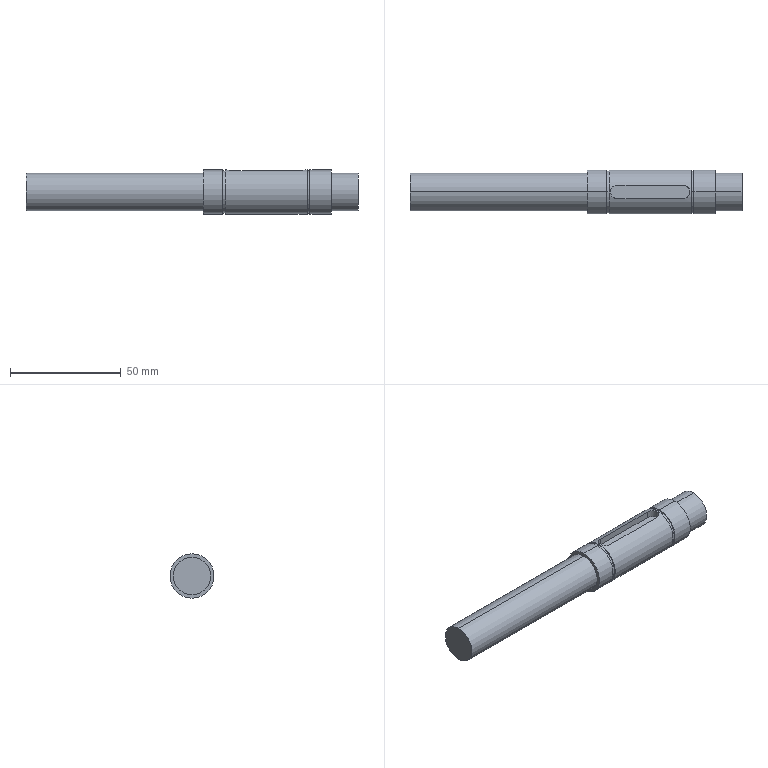Part | SolidWorks | features ICE 3, Extrusion 1, RevCut 1 | 1 solid | 28 faces | box 150 x 20 x 20 mm | volume 38325 mm3 | cylinder 17 | plane 11 | commonest cylinder face diameters 20 x6 17 x4 19 x4 6 x3
STEP:
#1=CARTESIAN_POINT('',(58.,0.,-10.));
#2=VERTEX_POINT('',#1);
#3=CARTESIAN_POINT('',(58.,0.,10.));
#4=VERTEX_POINT('',#3);
#5=CARTESIAN_POINT('',(58.,0.,0.));
#6=DIRECTION('',(1.,0.,0.));
#7=DIRECTION('',(0.,0.,-1.));
#8=AXIS2_PLACEMENT_3D('',#5,#6,#7);
#9=CIRCLE('',#8,10.);
#10=EDGE_CURVE('',#2,#4,#9,.T.);
#11=ORIENTED_EDGE('',*,*,#10,.F.);
#12=CARTESIAN_POINT('',(48.3,0.,-10.));
#13=VERTEX_POINT('',#12);
#14=CARTESIAN_POINT('',(58.,0.,-10.));
#15=DIRECTION('',(-1.,0.,0.));
#16=VECTOR('',#15,1000.);
#17=LINE('',#14,#16);
#18=EDGE_CURVE('',#2,#13,#17,.T.);
#19=ORIENTED_EDGE('',*,*,#18,.T.);
#20=CARTESIAN_POINT('',(48.3,0.,10.));
#21=VERTEX_POINT('',#20);
#22=CARTESIAN_POINT('',(48.3,0.,0.));
#23=DIRECTION('',(-1.,0.,0.));
#24=DIRECTION('',(0.,0.,1.));
#25=AXIS2_PLACEMENT_3D('',#22,#23,#24);
#26=CIRCLE('',#25,10.);
#27=EDGE_CURVE('',#21,#13,#26,.T.);
#28=ORIENTED_EDGE('',*,*,#27,.F.);
#29=CARTESIAN_POINT('',(58.,0.,10.));
#30=DIRECTION('',(-1.,0.,0.));
#31=VECTOR('',#30,1000.);
#32=LINE('',#29,#31);
#33=EDGE_CURVE('',#4,#21,#32,.T.);
#34=ORIENTED_EDGE('',*,*,#33,.F.);
#35=EDGE_LOOP('',(#11,#19,#28,#34));
#36=FACE_OUTER_BOUND('',#35,.T.);
#37=CARTESIAN_POINT('',(58.,0.,0.));
#38=DIRECTION('',(-1.,0.,0.));
#39=DIRECTION('',(0.,0.,1.));
#40=AXIS2_PLACEMENT_3D('',#37,#38,#39);
#41=CYLINDRICAL_SURFACE('',#40,10.);
#42=ADVANCED_FACE('',(#36),#41,.T.);
#43=CARTESIAN_POINT('',(70.,0.,-8.5));
#44=VERTEX_POINT('',#43);
#45=CARTESIAN_POINT('',(70.,0.,8.5));
#46=VERTEX_POINT('',#45);
#47=CARTESIAN_POINT('',(70.,0.,0.));
#48=DIRECTION('',(1.,0.,0.));
#49=DIRECTION('',(0.,0.,-1.));
#50=AXIS2_PLACEMENT_3D('',#47,#48,#49);
#51=CIRCLE('',#50,8.5);
#52=EDGE_CURVE('',#44,#46,#51,.T.);
#53=ORIENTED_EDGE('',*,*,#52,.F.);
#54=CARTESIAN_POINT('',(58.,0.,-8.5));
#55=VERTEX_POINT('',#54);
#56=CARTESIAN_POINT('',(70.,0.,-8.5));
#57=DIRECTION('',(-1.,0.,0.));
#58=VECTOR('',#57,1000.);
#59=LINE('',#56,#58);
#60=EDGE_CURVE('',#44,#55,#59,.T.);
#61=ORIENTED_EDGE('',*,*,#60,.T.);
#62=CARTESIAN_POINT('',(58.,0.,8.5));
#63=VERTEX_POINT('',#62);
#64=CARTESIAN_POINT('',(58.,0.,0.));
#65=DIRECTION('',(1.,0.,0.));
#66=DIRECTION('',(0.,0.,-1.));
#67=AXIS2_PLACEMENT_3D('',#64,#65,#66);
#68=CIRCLE('',#67,8.5);
#69=EDGE_CURVE('',#55,#63,#68,.T.);
#70=ORIENTED_EDGE('',*,*,#69,.T.);
#71=CARTESIAN_POINT('',(70.,0.,8.5));
#72=DIRECTION('',(-1.,0.,0.));
#73=VECTOR('',#72,1000.);
#74=LINE('',#71,#73);
#75=EDGE_CURVE('',#46,#63,#74,.T.);
#76=ORIENTED_EDGE('',*,*,#75,.F.);
#77=EDGE_LOOP('',(#53,#61,#70,#76));
#78=FACE_OUTER_BOUND('',#77,.T.);
#79=CARTESIAN_POINT('',(70.,0.,0.));
#80=DIRECTION('',(-1.,0.,0.));
#81=DIRECTION('',(0.,0.,1.));
#82=AXIS2_PLACEMENT_3D('',#79,#80,#81);
#83=CYLINDRICAL_SURFACE('',#82,8.5);
#84=ADVANCED_FACE('',(#78),#83,.T.);
#85=CARTESIAN_POINT('',(48.3,0.,9.5));
#86=VERTEX_POINT('',#85);
#87=CARTESIAN_POINT('',(48.3,0.,-9.5));
#88=VERTEX_POINT('',#87);
#89=CARTESIAN_POINT('',(48.3,0.,0.));
#90=DIRECTION('',(-1.,0.,0.));
#91=DIRECTION('',(0.,0.,1.));
#92=AXIS2_PLACEMENT_3D('',#89,#90,#91);
#93=CIRCLE('',#92,9.5);
#94=EDGE_CURVE('',#86,#88,#93,.T.);
#95=ORIENTED_EDGE('',*,*,#94,.T.);
#96=CARTESIAN_POINT('',(47.,0.,-9.5));
#97=VERTEX_POINT('',#96);
#98=CARTESIAN_POINT('',(0.,0.,-9.5));
#99=DIRECTION('',(-1.,0.,0.));
#100=VECTOR('',#99,1000.);
#101=LINE('',#98,#100);
#102=EDGE_CURVE('',#88,#97,#101,.T.);
#103=ORIENTED_EDGE('',*,*,#102,.T.);
#104=CARTESIAN_POINT('',(47.,0.,9.5));
#105=VERTEX_POINT('',#104);
#106=CARTESIAN_POINT('',(47.,0.,0.));
#107=DIRECTION('',(-1.,0.,0.));
#108=DIRECTION('',(0.,0.,1.));
#109=AXIS2_PLACEMENT_3D('',#106,#107,#108);
#110=CIRCLE('',#109,9.5);
#111=EDGE_CURVE('',#105,#97,#110,.T.);
#112=ORIENTED_EDGE('',*,*,#111,.F.);
#113=CARTESIAN_POINT('',(0.,0.,9.5));
#114=DIRECTION('',(-1.,0.,0.));
#115=VECTOR('',#114,1000.);
#116=LINE('',#113,#115);
#117=EDGE_CURVE('',#86,#105,#116,.T.);
#118=ORIENTED_EDGE('',*,*,#117,.F.);
#119=EDGE_LOOP('',(#95,#103,#112,#118));
#120=FACE_OUTER_BOUND('',#119,.T.);
#121=CARTESIAN_POINT('',(0.,0.,0.));
#122=DIRECTION('',(-1.,0.,0.));
#123=DIRECTION('',(0.,0.,1.));
#124=AXIS2_PLACEMENT_3D('',#121,#122,#123);
#125=CYLINDRICAL_SURFACE('',#124,9.5);
#126=ADVANCED_FACE('',(#120),#125,.T.);
#127=CARTESIAN_POINT('',(47.,0.,10.));
#128=VERTEX_POINT('',#127);
#129=CARTESIAN_POINT('',(47.,0.,-10.));
#130=VERTEX_POINT('',#129);
#131=CARTESIAN_POINT('',(47.,0.,0.));
#132=DIRECTION('',(-1.,0.,0.));
#133=DIRECTION('',(0.,0.,1.));
#134=AXIS2_PLACEMENT_3D('',#131,#132,#133);
#135=CIRCLE('',#134,10.);
#136=EDGE_CURVE('',#128,#130,#135,.T.);
#137=ORIENTED_EDGE('',*,*,#136,.T.);
#138=CARTESIAN_POINT('',(10.,0.,-10.));
#139=VERTEX_POINT('',#138);
#140=CARTESIAN_POINT('',(58.,0.,-10.));
#141=DIRECTION('',(-1.,0.,0.));
#142=VECTOR('',#141,1000.);
#143=LINE('',#140,#142);
#144=EDGE_CURVE('',#130,#139,#143,.T.);
#145=ORIENTED_EDGE('',*,*,#144,.T.);
#146=CARTESIAN_POINT('',(10.,0.,10.));
#147=VERTEX_POINT('',#146);
#148=CARTESIAN_POINT('',(10.,0.,0.));
#149=DIRECTION('',(-1.,0.,0.));
#150=DIRECTION('',(0.,0.,1.));
#151=AXIS2_PLACEMENT_3D('',#148,#149,#150);
#152=CIRCLE('',#151,10.);
#153=EDGE_CURVE('',#147,#139,#152,.T.);
#154=ORIENTED_EDGE('',*,*,#153,.F.);
#155=CARTESIAN_POINT('',(10.5,0.,10.));
#156=VERTEX_POINT('',#155);
#157=CARTESIAN_POINT('',(58.,0.,10.));
#158=DIRECTION('',(-1.,0.,0.));
#159=VECTOR('',#158,1000.);
#160=LINE('',#157,#159);
#161=EDGE_CURVE('',#156,#147,#160,.T.);
#162=ORIENTED_EDGE('',*,*,#161,.F.);
#163=CARTESIAN_POINT('',(13.5,3.,9.539));
#164=VERTEX_POINT('',#163);
#165=CARTESIAN_POINT('',(13.5,3.,9.539));
#166=CARTESIAN_POINT('',(13.3,3.,9.539));
#167=CARTESIAN_POINT('',(13.105,2.98,9.546));
#168=CARTESIAN_POINT('',(12.719,2.903,9.569));
#169=CARTESIAN_POINT('',(12.528,2.845,9.587));
#170=CARTESIAN_POINT('',(12.165,2.694,9.631));
#171=CARTESIAN_POINT('',(11.994,2.602,9.656));
#172=CARTESIAN_POINT('',(11.668,2.384,9.712));
#173=CARTESIAN_POINT('',(11.515,2.258,9.743));
#174=CARTESIAN_POINT('',(11.103,1.845,9.832));
#175=CARTESIAN_POINT('',(10.88,1.512,9.892));
#176=CARTESIAN_POINT('',(10.655,0.971,9.954));
#177=CARTESIAN_POINT('',(10.597,0.7806,9.971));
#178=CARTESIAN_POINT('',(10.519,0.3926,9.994));
#179=CARTESIAN_POINT('',(10.5,0.197,10.));
#180=CARTESIAN_POINT('',(10.5,0.,10.));
#181=B_SPLINE_CURVE_WITH_KNOTS('',3,(#165,#166,#167,#168,#169,#170,#171,#172,#173,#174,#175,#176,#177,#178,#179,#180),.UNSPECIFIED.,.F.,.F.,(4,2,2,2,2,2,2,4),(0.,0.0005898,0.00118,0.001769,0.002359,0.003539,0.004128,0.004718),.UNSPECIFIED.);
#182=EDGE_CURVE('',#164,#156,#181,.T.);
#183=ORIENTED_EDGE('',*,*,#182,.F.);
#184=CARTESIAN_POINT('',(43.5,3.,9.539));
#185=VERTEX_POINT('',#184);
#186=CARTESIAN_POINT('',(58.,3.,9.539));
#187=DIRECTION('',(-1.,0.,0.));
#188=VECTOR('',#187,1000.);
#189=LINE('',#186,#188);
#190=EDGE_CURVE('',#185,#164,#189,.T.);
#191=ORIENTED_EDGE('',*,*,#190,.F.);
#192=CARTESIAN_POINT('',(46.5,0.,10.));
#193=VERTEX_POINT('',#192);
#194=CARTESIAN_POINT('',(46.5,0.,10.));
#195=CARTESIAN_POINT('',(46.5,0.1968,10.));
#196=CARTESIAN_POINT('',(46.48,0.3967,9.994));
#197=CARTESIAN_POINT('',(46.403,0.7821,9.971));
#198=CARTESIAN_POINT('',(46.346,0.9695,9.955));
#199=CARTESIAN_POINT('',(46.194,1.334,9.912));
#200=CARTESIAN_POINT('',(46.101,1.507,9.887));
#201=CARTESIAN_POINT('',(45.884,1.831,9.832));
#202=CARTESIAN_POINT('',(45.759,1.983,9.802));
#203=CARTESIAN_POINT('',(45.483,2.26,9.742));
#204=CARTESIAN_POINT('',(45.333,2.383,9.713));
#205=CARTESIAN_POINT('',(45.009,2.6,9.657));
#206=CARTESIAN_POINT('',(44.833,2.694,9.63));
#207=CARTESIAN_POINT('',(44.472,2.845,9.587));
#208=CARTESIAN_POINT('',(44.285,2.902,9.57));
#209=CARTESIAN_POINT('',(43.899,2.98,9.546));
#210=CARTESIAN_POINT('',(43.699,3.,9.539));
#211=CARTESIAN_POINT('',(43.5,3.,9.539));
#212=B_SPLINE_CURVE_WITH_KNOTS('',3,(#194,#195,#196,#197,#198,#199,#200,#201,#202,#203,#204,#205,#206,#207,#208,#209,#210,#211),.UNSPECIFIED.,.F.,.F.,(4,2,2,2,2,2,2,2,4),(0.004718,0.005307,0.005896,0.006485,0.007074,0.007663,0.008252,0.008842,0.009431),.UNSPECIFIED.);
#213=EDGE_CURVE('',#193,#185,#212,.T.);
#214=ORIENTED_EDGE('',*,*,#213,.F.);
#215=CARTESIAN_POINT('',(58.,0.,10.));
#216=DIRECTION('',(-1.,0.,0.));
#217=VECTOR('',#216,1000.);
#218=LINE('',#215,#217);
#219=EDGE_CURVE('',#128,#193,#218,.T.);
#220=ORIENTED_EDGE('',*,*,#219,.F.);
#221=EDGE_LOOP('',(#137,#145,#154,#162,#183,#191,#214,#220));
#222=FACE_OUTER_BOUND('',#221,.T.);
#223=CARTESIAN_POINT('',(58.,0.,0.));
#224=DIRECTION('',(-1.,0.,0.));
#225=DIRECTION('',(0.,0.,1.));
#226=AXIS2_PLACEMENT_3D('',#223,#224,#225);
#227=CYLINDRICAL_SURFACE('',#226,10.);
#228=ADVANCED_FACE('',(#222),#227,.T.);
#229=ORIENTED_EDGE('',*,*,#182,.T.);
#230=CARTESIAN_POINT('',(10.5,0.,6.5));
#231=VERTEX_POINT('',#230);
#232=CARTESIAN_POINT('',(10.5,0.,10.));
#233=DIRECTION('',(0.,0.,-1.));
#234=VECTOR('',#233,1000.);
#235=LINE('',#232,#234);
#236=EDGE_CURVE('',#156,#231,#235,.T.);
#237=ORIENTED_EDGE('',*,*,#236,.T.);
#238=CARTESIAN_POINT('',(13.5,3.,6.5));
#239=VERTEX_POINT('',#238);
#240=CARTESIAN_POINT('',(13.5,0.,6.5));
#241=DIRECTION('',(0.,0.,1.));
#242=DIRECTION('',(1.,0.,0.));
#243=AXIS2_PLACEMENT_3D('',#240,#241,#242);
#244=CIRCLE('',#243,3.);
#245=EDGE_CURVE('',#239,#231,#244,.T.);
#246=ORIENTED_EDGE('',*,*,#245,.F.);
#247=CARTESIAN_POINT('',(13.5,3.,10.));
#248=DIRECTION('',(0.,0.,-1.));
#249=VECTOR('',#248,1000.);
#250=LINE('',#247,#249);
#251=EDGE_CURVE('',#164,#239,#250,.T.);
#252=ORIENTED_EDGE('',*,*,#251,.F.);
#253=EDGE_LOOP('',(#229,#237,#246,#252));
#254=FACE_OUTER_BOUND('',#253,.T.);
#255=CARTESIAN_POINT('',(13.5,0.,10.));
#256=DIRECTION('',(0.,0.,-1.));
#257=DIRECTION('',(-1.,0.,0.));
#258=AXIS2_PLACEMENT_3D('',#255,#256,#257);
#259=CYLINDRICAL_SURFACE('',#258,3.);
#260=ADVANCED_FACE('',(#254),#259,.F.);
#261=CARTESIAN_POINT('',(10.,0.,9.5));
#262=VERTEX_POINT('',#261);
#263=CARTESIAN_POINT('',(10.,0.,-9.5));
#264=VERTEX_POINT('',#263);
#265=CARTESIAN_POINT('',(10.,0.,0.));
#266=DIRECTION('',(-1.,0.,0.));
#267=DIRECTION('',(0.,0.,1.));
#268=AXIS2_PLACEMENT_3D('',#265,#266,#267);
#269=CIRCLE('',#268,9.5);
#270=EDGE_CURVE('',#262,#264,#269,.T.);
#271=ORIENTED_EDGE('',*,*,#270,.T.);
#272=CARTESIAN_POINT('',(8.7,0.,-9.5));
#273=VERTEX_POINT('',#272);
#274=CARTESIAN_POINT('',(0.,0.,-9.5));
#275=DIRECTION('',(-1.,0.,0.));
#276=VECTOR('',#275,1000.);
#277=LINE('',#274,#276);
#278=EDGE_CURVE('',#264,#273,#277,.T.);
#279=ORIENTED_EDGE('',*,*,#278,.T.);
#280=CARTESIAN_POINT('',(8.7,0.,9.5));
#281=VERTEX_POINT('',#280);
#282=CARTESIAN_POINT('',(8.7,0.,0.));
#283=DIRECTION('',(-1.,0.,0.));
#284=DIRECTION('',(0.,0.,1.));
#285=AXIS2_PLACEMENT_3D('',#282,#283,#284);
#286=CIRCLE('',#285,9.5);
#287=EDGE_CURVE('',#281,#273,#286,.T.);
#288=ORIENTED_EDGE('',*,*,#287,.F.);
#289=CARTESIAN_POINT('',(0.,0.,9.5));
#290=DIRECTION('',(-1.,0.,0.));
#291=VECTOR('',#290,1000.);
#292=LINE('',#289,#291);
#293=EDGE_CURVE('',#262,#281,#292,.T.);
#294=ORIENTED_EDGE('',*,*,#293,.F.);
#295=EDGE_LOOP('',(#271,#279,#288,#294));
#296=FACE_OUTER_BOUND('',#295,.T.);
#297=CARTESIAN_POINT('',(0.,0.,0.));
#298=DIRECTION('',(-1.,0.,0.));
#299=DIRECTION('',(0.,0.,1.));
#300=AXIS2_PLACEMENT_3D('',#297,#298,#299);
#301=CYLINDRICAL_SURFACE('',#300,9.5);
#302=ADVANCED_FACE('',(#296),#301,.T.);
#303=CARTESIAN_POINT('',(-80.,0.,8.5));
#304=VERTEX_POINT('',#303);
#305=CARTESIAN_POINT('',(-80.,0.,-8.5));
#306=VERTEX_POINT('',#305);
#307=CARTESIAN_POINT('',(-80.,0.,0.));
#308=DIRECTION('',(-1.,0.,0.));
#309=DIRECTION('',(0.,0.,1.));
#310=AXIS2_PLACEMENT_3D('',#307,#308,#309);
#311=CIRCLE('',#310,8.5);
#312=EDGE_CURVE('',#304,#306,#311,.T.);
#313=ORIENTED_EDGE('',*,*,#312,.F.);
#314=CARTESIAN_POINT('',(0.,0.,8.5));
#315=VERTEX_POINT('',#314);
#316=CARTESIAN_POINT('',(-80.,0.,8.5));
#317=DIRECTION('',(1.,0.,0.));
#318=VECTOR('',#317,1000.);
#319=LINE('',#316,#318);
#320=EDGE_CURVE('',#304,#315,#319,.T.);
#321=ORIENTED_EDGE('',*,*,#320,.T.);
#322=CARTESIAN_POINT('',(0.,0.,-8.5));
#323=VERTEX_POINT('',#322);
#324=CARTESIAN_POINT('',(0.,0.,0.));
#325=DIRECTION('',(-1.,0.,0.));
#326=DIRECTION('',(0.,0.,1.));
#327=AXIS2_PLACEMENT_3D('',#324,#325,#326);
#328=CIRCLE('',#327,8.5);
#329=EDGE_CURVE('',#315,#323,#328,.T.);
#330=ORIENTED_EDGE('',*,*,#329,.T.);
#331=CARTESIAN_POINT('',(-80.,0.,-8.5));
#332=DIRECTION('',(1.,0.,0.));
#333=VECTOR('',#332,1000.);
#334=LINE('',#331,#333);
#335=EDGE_CURVE('',#306,#323,#334,.T.);
#336=ORIENTED_EDGE('',*,*,#335,.F.);
#337=EDGE_LOOP('',(#313,#321,#330,#336));
#338=FACE_OUTER_BOUND('',#337,.T.);
#339=CARTESIAN_POINT('',(-80.,0.,0.));
#340=DIRECTION('',(1.,0.,0.));
#341=DIRECTION('',(0.,0.,-1.));
#342=AXIS2_PLACEMENT_3D('',#339,#340,#341);
#343=CYLINDRICAL_SURFACE('',#342,8.5);
#344=ADVANCED_FACE('',(#338),#343,.T.);
#345=CARTESIAN_POINT('',(8.7,0.,10.));
#346=VERTEX_POINT('',#345);
#347=CARTESIAN_POINT('',(8.7,0.,-10.));
#348=VERTEX_POINT('',#347);
#349=CARTESIAN_POINT('',(8.7,0.,0.));
#350=DIRECTION('',(-1.,0.,0.));
#351=DIRECTION('',(0.,0.,1.));
#352=AXIS2_PLACEMENT_3D('',#349,#350,#351);
#353=CIRCLE('',#352,10.);
#354=EDGE_CURVE('',#346,#348,#353,.T.);
#355=ORIENTED_EDGE('',*,*,#354,.T.);
#356=CARTESIAN_POINT('',(0.,0.,-10.));
#357=VERTEX_POINT('',#356);
#358=CARTESIAN_POINT('',(58.,0.,-10.));
#359=DIRECTION('',(-1.,0.,0.));
#360=VECTOR('',#359,1000.);
#361=LINE('',#358,#360);
#362=EDGE_CURVE('',#348,#357,#361,.T.);
#363=ORIENTED_EDGE('',*,*,#362,.T.);
#364=CARTESIAN_POINT('',(0.,0.,10.));
#365=VERTEX_POINT('',#364);
#366=CARTESIAN_POINT('',(0.,0.,0.));
#367=DIRECTION('',(1.,0.,0.));
#368=DIRECTION('',(0.,0.,-1.));
#369=AXIS2_PLACEMENT_3D('',#366,#367,#368);
#370=CIRCLE('',#369,10.);
#371=EDGE_CURVE('',#357,#365,#370,.T.);
#372=ORIENTED_EDGE('',*,*,#371,.T.);
#373=CARTESIAN_POINT('',(58.,0.,10.));
#374=DIRECTION('',(-1.,0.,0.));
#375=VECTOR('',#374,1000.);
#376=LINE('',#373,#375);
#377=EDGE_CURVE('',#346,#365,#376,.T.);
#378=ORIENTED_EDGE('',*,*,#377,.F.);
#379=EDGE_LOOP('',(#355,#363,#372,#378));
#380=FACE_OUTER_BOUND('',#379,.T.);
#381=CARTESIAN_POINT('',(58.,0.,0.));
#382=DIRECTION('',(-1.,0.,0.));
#383=DIRECTION('',(0.,0.,1.));
#384=AXIS2_PLACEMENT_3D('',#381,#382,#383);
#385=CYLINDRICAL_SURFACE('',#384,10.);
#386=ADVANCED_FACE('',(#380),#385,.T.);
#387=ORIENTED_EDGE('',*,*,#362,.F.);
#388=CARTESIAN_POINT('',(8.7,0.,0.));
#389=DIRECTION('',(-1.,0.,0.));
#390=DIRECTION('',(0.,0.,1.));
#391=AXIS2_PLACEMENT_3D('',#388,#389,#390);
#392=CIRCLE('',#391,10.);
#393=EDGE_CURVE('',#348,#346,#392,.T.);
#394=ORIENTED_EDGE('',*,*,#393,.T.);
#395=ORIENTED_EDGE('',*,*,#377,.T.);
#396=CARTESIAN_POINT('',(0.,0.,0.));
#397=DIRECTION('',(1.,0.,0.));
#398=DIRECTION('',(0.,0.,-1.));
#399=AXIS2_PLACEMENT_3D('',#396,#397,#398);
#400=CIRCLE('',#399,10.);
#401=EDGE_CURVE('',#365,#357,#400,.T.);
#402=ORIENTED_EDGE('',*,*,#401,.T.);
#403=EDGE_LOOP('',(#387,#394,#395,#402));
#404=FACE_OUTER_BOUND('',#403,.T.);
#405=CARTESIAN_POINT('',(58.,0.,0.));
#406=DIRECTION('',(-1.,0.,0.));
#407=DIRECTION('',(0.,0.,1.));
#408=AXIS2_PLACEMENT_3D('',#405,#406,#407);
#409=CYLINDRICAL_SURFACE('',#408,10.);
#410=ADVANCED_FACE('',(#404),#409,.T.);
#411=CARTESIAN_POINT('',(0.,0.,0.));
#412=DIRECTION('',(-1.,0.,0.));
#413=DIRECTION('',(0.,0.,1.));
#414=AXIS2_PLACEMENT_3D('',#411,#412,#413);
#415=CIRCLE('',#414,8.5);
#416=EDGE_CURVE('',#323,#315,#415,.T.);
#417=ORIENTED_EDGE('',*,*,#416,.F.);
#418=ORIENTED_EDGE('',*,*,#329,.F.);
#419=EDGE_LOOP('',(#417,#418));
#420=FACE_BOUND('',#419,.T.);
#421=ORIENTED_EDGE('',*,*,#401,.F.);
#422=ORIENTED_EDGE('',*,*,#371,.F.);
#423=EDGE_LOOP('',(#421,#422));
#424=FACE_OUTER_BOUND('',#423,.T.);
#425=CARTESIAN_POINT('',(0.,0.,0.));
#426=DIRECTION('',(1.,0.,0.));
#427=DIRECTION('',(0.,0.,-1.));
#428=AXIS2_PLACEMENT_3D('',#425,#426,#427);
#429=PLANE('',#428);
#430=ADVANCED_FACE('',(#420,#424),#429,.F.);
#431=ORIENTED_EDGE('',*,*,#320,.F.);
#432=CARTESIAN_POINT('',(-80.,0.,0.));
#433=DIRECTION('',(-1.,0.,0.));
#434=DIRECTION('',(0.,0.,1.));
#435=AXIS2_PLACEMENT_3D('',#432,#433,#434);
#436=CIRCLE('',#435,8.5);
#437=EDGE_CURVE('',#306,#304,#436,.T.);
#438=ORIENTED_EDGE('',*,*,#437,.F.);
#439=ORIENTED_EDGE('',*,*,#335,.T.);
#440=ORIENTED_EDGE('',*,*,#416,.T.);
#441=EDGE_LOOP('',(#431,#438,#439,#440));
#442=FACE_OUTER_BOUND('',#441,.T.);
#443=CARTESIAN_POINT('',(-80.,0.,0.));
#444=DIRECTION('',(1.,0.,0.));
#445=DIRECTION('',(0.,0.,-1.));
#446=AXIS2_PLACEMENT_3D('',#443,#444,#445);
#447=CYLINDRICAL_SURFACE('',#446,8.5);
#448=ADVANCED_FACE('',(#442),#447,.T.);
#449=ORIENTED_EDGE('',*,*,#437,.T.);
#450=ORIENTED_EDGE('',*,*,#312,.T.);
#451=EDGE_LOOP('',(#449,#450));
#452=FACE_OUTER_BOUND('',#451,.T.);
#453=CARTESIAN_POINT('',(-80.,0.,0.));
#454=DIRECTION('',(-1.,0.,0.));
#455=DIRECTION('',(0.,0.,1.));
#456=AXIS2_PLACEMENT_3D('',#453,#454,#455);
#457=PLANE('',#456);
#458=ADVANCED_FACE('',(#452),#457,.T.);
#459=ORIENTED_EDGE('',*,*,#287,.T.);
#460=CARTESIAN_POINT('',(8.7,0.,0.));
#461=DIRECTION('',(-1.,0.,0.));
#462=DIRECTION('',(0.,0.,1.));
#463=AXIS2_PLACEMENT_3D('',#460,#461,#462);
#464=CIRCLE('',#463,9.5);
#465=EDGE_CURVE('',#273,#281,#464,.T.);
#466=ORIENTED_EDGE('',*,*,#465,.T.);
#467=EDGE_LOOP('',(#459,#466));
#468=FACE_BOUND('',#467,.T.);
#469=ORIENTED_EDGE('',*,*,#354,.F.);
#470=ORIENTED_EDGE('',*,*,#393,.F.);
#471=EDGE_LOOP('',(#469,#470));
#472=FACE_OUTER_BOUND('',#471,.T.);
#473=CARTESIAN_POINT('',(8.7,0.,-10.));
#474=DIRECTION('',(1.,0.,0.));
#475=DIRECTION('',(0.,0.,-1.));
#476=AXIS2_PLACEMENT_3D('',#473,#474,#475);
#477=PLANE('',#476);
#478=ADVANCED_FACE('',(#468,#472),#477,.T.);
#479=ORIENTED_EDGE('',*,*,#278,.F.);
#480=CARTESIAN_POINT('',(10.,0.,0.));
#481=DIRECTION('',(-1.,0.,0.));
#482=DIRECTION('',(0.,0.,1.));
#483=AXIS2_PLACEMENT_3D('',#480,#481,#482);
#484=CIRCLE('',#483,9.5);
#485=EDGE_CURVE('',#264,#262,#484,.T.);
#486=ORIENTED_EDGE('',*,*,#485,.T.);
#487=ORIENTED_EDGE('',*,*,#293,.T.);
#488=ORIENTED_EDGE('',*,*,#465,.F.);
#489=EDGE_LOOP('',(#479,#486,#487,#488));
#490=FACE_OUTER_BOUND('',#489,.T.);
#491=CARTESIAN_POINT('',(0.,0.,0.));
#492=DIRECTION('',(-1.,0.,0.));
#493=DIRECTION('',(0.,0.,1.));
#494=AXIS2_PLACEMENT_3D('',#491,#492,#493);
#495=CYLINDRICAL_SURFACE('',#494,9.5);
#496=ADVANCED_FACE('',(#490),#495,.T.);
#497=ORIENTED_EDGE('',*,*,#153,.T.);
#498=CARTESIAN_POINT('',(10.,0.,0.));
#499=DIRECTION('',(-1.,0.,0.));
#500=DIRECTION('',(0.,0.,1.));
#501=AXIS2_PLACEMENT_3D('',#498,#499,#500);
#502=CIRCLE('',#501,10.);
#503=EDGE_CURVE('',#139,#147,#502,.T.);
#504=ORIENTED_EDGE('',*,*,#503,.T.);
#505=EDGE_LOOP('',(#497,#504));
#506=FACE_OUTER_BOUND('',#505,.T.);
#507=ORIENTED_EDGE('',*,*,#270,.F.);
#508=ORIENTED_EDGE('',*,*,#485,.F.);
#509=EDGE_LOOP('',(#507,#508));
#510=FACE_BOUND('',#509,.T.);
#511=CARTESIAN_POINT('',(10.,0.,-10.));
#512=DIRECTION('',(-1.,0.,0.));
#513=DIRECTION('',(0.,0.,1.));
#514=AXIS2_PLACEMENT_3D('',#511,#512,#513);
#515=PLANE('',#514);
#516=ADVANCED_FACE('',(#506,#510),#515,.T.);
#517=ORIENTED_EDGE('',*,*,#245,.T.);
#518=CARTESIAN_POINT('',(13.5,-3.,6.5));
#519=VERTEX_POINT('',#518);
#520=CARTESIAN_POINT('',(13.5,0.,6.5));
#521=DIRECTION('',(0.,0.,1.));
#522=DIRECTION('',(1.,0.,0.));
#523=AXIS2_PLACEMENT_3D('',#520,#521,#522);
#524=CIRCLE('',#523,3.);
#525=EDGE_CURVE('',#231,#519,#524,.T.);
#526=ORIENTED_EDGE('',*,*,#525,.T.);
#527=CARTESIAN_POINT('',(43.5,-3.,6.5));
#528=VERTEX_POINT('',#527);
#529=CARTESIAN_POINT('',(13.5,-3.,6.5));
#530=DIRECTION('',(1.,0.,0.));
#531=VECTOR('',#530,1000.);
#532=LINE('',#529,#531);
#533=EDGE_CURVE('',#519,#528,#532,.T.);
#534=ORIENTED_EDGE('',*,*,#533,.T.);
#535=CARTESIAN_POINT('',(43.5,3.,6.5));
#536=VERTEX_POINT('',#535);
#537=CARTESIAN_POINT('',(43.5,0.,6.5));
#538=DIRECTION('',(0.,0.,1.));
#539=DIRECTION('',(1.,0.,0.));
#540=AXIS2_PLACEMENT_3D('',#537,#538,#539);
#541=CIRCLE('',#540,3.);
#542=EDGE_CURVE('',#528,#536,#541,.T.);
#543=ORIENTED_EDGE('',*,*,#542,.T.);
#544=CARTESIAN_POINT('',(13.5,3.,6.5));
#545=DIRECTION('',(-1.,0.,0.));
#546=VECTOR('',#545,1000.);
#547=LINE('',#544,#546);
#548=EDGE_CURVE('',#536,#239,#547,.T.);
#549=ORIENTED_EDGE('',*,*,#548,.T.);
#550=EDGE_LOOP('',(#517,#526,#534,#543,#549));
#551=FACE_OUTER_BOUND('',#550,.T.);
#552=CARTESIAN_POINT('',(13.5,0.,6.5));
#553=DIRECTION('',(0.,0.,1.));
#554=DIRECTION('',(1.,0.,0.));
#555=AXIS2_PLACEMENT_3D('',#552,#553,#554);
#556=PLANE('',#555);
#557=ADVANCED_FACE('',(#551),#556,.T.);
#558=ORIENTED_EDGE('',*,*,#190,.T.);
#559=ORIENTED_EDGE('',*,*,#251,.T.);
#560=ORIENTED_EDGE('',*,*,#548,.F.);
#561=CARTESIAN_POINT('',(43.5,3.,10.));
#562=DIRECTION('',(0.,0.,-1.));
#563=VECTOR('',#562,1000.);
#564=LINE('',#561,#563);
#565=EDGE_CURVE('',#185,#536,#564,.T.);
#566=ORIENTED_EDGE('',*,*,#565,.F.);
#567=EDGE_LOOP('',(#558,#559,#560,#566));
#568=FACE_OUTER_BOUND('',#567,.T.);
#569=CARTESIAN_POINT('',(13.5,3.,10.));
#570=DIRECTION('',(0.,-1.,0.));
#571=DIRECTION('',(1.,0.,0.));
#572=AXIS2_PLACEMENT_3D('',#569,#570,#571);
#573=PLANE('',#572);
#574=ADVANCED_FACE('',(#568),#573,.T.);
#575=ORIENTED_EDGE('',*,*,#236,.F.);
#576=CARTESIAN_POINT('',(13.5,-3.,9.539));
#577=VERTEX_POINT('',#576);
#578=CARTESIAN_POINT('',(10.5,0.,10.));
#579=CARTESIAN_POINT('',(10.5,-0.1968,10.));
#580=CARTESIAN_POINT('',(10.52,-0.3967,9.994));
#581=CARTESIAN_POINT('',(10.597,-0.7821,9.971));
#582=CARTESIAN_POINT('',(10.654,-0.9695,9.955));
#583=CARTESIAN_POINT('',(10.806,-1.334,9.912));
#584=CARTESIAN_POINT('',(10.899,-1.507,9.887));
#585=CARTESIAN_POINT('',(11.116,-1.831,9.832));
#586=CARTESIAN_POINT('',(11.241,-1.983,9.802));
#587=CARTESIAN_POINT('',(11.517,-2.26,9.742));
#588=CARTESIAN_POINT('',(11.667,-2.383,9.713));
#589=CARTESIAN_POINT('',(11.991,-2.6,9.657));
#590=CARTESIAN_POINT('',(12.167,-2.694,9.63));
#591=CARTESIAN_POINT('',(12.528,-2.845,9.587));
#592=CARTESIAN_POINT('',(12.715,-2.902,9.57));
#593=CARTESIAN_POINT('',(13.101,-2.98,9.546));
#594=CARTESIAN_POINT('',(13.301,-3.,9.539));
#595=CARTESIAN_POINT('',(13.5,-3.,9.539));
#596=B_SPLINE_CURVE_WITH_KNOTS('',3,(#578,#579,#580,#581,#582,#583,#584,#585,#586,#587,#588,#589,#590,#591,#592,#593,#594,#595),.UNSPECIFIED.,.F.,.F.,(4,2,2,2,2,2,2,2,4),(0.004718,0.005307,0.005896,0.006485,0.007074,0.007663,0.008252,0.008842,0.009431),.UNSPECIFIED.);
#597=EDGE_CURVE('',#156,#577,#596,.T.);
#598=ORIENTED_EDGE('',*,*,#597,.T.);
#599=CARTESIAN_POINT('',(13.5,-3.,10.));
#600=DIRECTION('',(0.,0.,-1.));
#601=VECTOR('',#600,1000.);
#602=LINE('',#599,#601);
#603=EDGE_CURVE('',#577,#519,#602,.T.);
#604=ORIENTED_EDGE('',*,*,#603,.T.);
#605=ORIENTED_EDGE('',*,*,#525,.F.);
#606=EDGE_LOOP('',(#575,#598,#604,#605));
#607=FACE_OUTER_BOUND('',#606,.T.);
#608=CARTESIAN_POINT('',(13.5,0.,10.));
#609=DIRECTION('',(0.,0.,-1.));
#610=DIRECTION('',(-1.,0.,0.));
#611=AXIS2_PLACEMENT_3D('',#608,#609,#610);
#612=CYLINDRICAL_SURFACE('',#611,3.);
#613=ADVANCED_FACE('',(#607),#612,.F.);
#614=CARTESIAN_POINT('',(43.5,-3.,9.539));
#615=VERTEX_POINT('',#614);
#616=CARTESIAN_POINT('',(58.,-3.,9.539));
#617=DIRECTION('',(1.,0.,0.));
#618=VECTOR('',#617,1000.);
#619=LINE('',#616,#618);
#620=EDGE_CURVE('',#577,#615,#619,.T.);
#621=ORIENTED_EDGE('',*,*,#620,.T.);
#622=CARTESIAN_POINT('',(43.5,-3.,10.));
#623=DIRECTION('',(0.,0.,-1.));
#624=VECTOR('',#623,1000.);
#625=LINE('',#622,#624);
#626=EDGE_CURVE('',#615,#528,#625,.T.);
#627=ORIENTED_EDGE('',*,*,#626,.T.);
#628=ORIENTED_EDGE('',*,*,#533,.F.);
#629=ORIENTED_EDGE('',*,*,#603,.F.);
#630=EDGE_LOOP('',(#621,#627,#628,#629));
#631=FACE_OUTER_BOUND('',#630,.T.);
#632=CARTESIAN_POINT('',(13.5,-3.,10.));
#633=DIRECTION('',(0.,1.,0.));
#634=DIRECTION('',(-1.,0.,0.));
#635=AXIS2_PLACEMENT_3D('',#632,#633,#634);
#636=PLANE('',#635);
#637=ADVANCED_FACE('',(#631),#636,.T.);
#638=ORIENTED_EDGE('',*,*,#626,.F.);
#639=CARTESIAN_POINT('',(43.5,-3.,9.539));
#640=CARTESIAN_POINT('',(43.7,-3.,9.539));
#641=CARTESIAN_POINT('',(43.895,-2.98,9.546));
#642=CARTESIAN_POINT('',(44.281,-2.903,9.569));
#643=CARTESIAN_POINT('',(44.472,-2.845,9.587));
#644=CARTESIAN_POINT('',(44.835,-2.694,9.631));
#645=CARTESIAN_POINT('',(45.006,-2.602,9.656));
#646=CARTESIAN_POINT('',(45.332,-2.384,9.712));
#647=CARTESIAN_POINT('',(45.485,-2.258,9.743));
#648=CARTESIAN_POINT('',(45.897,-1.845,9.832));
#649=CARTESIAN_POINT('',(46.12,-1.512,9.892));
#650=CARTESIAN_POINT('',(46.345,-0.971,9.954));
#651=CARTESIAN_POINT('',(46.403,-0.7806,9.971));
#652=CARTESIAN_POINT('',(46.481,-0.3926,9.994));
#653=CARTESIAN_POINT('',(46.5,-0.197,10.));
#654=CARTESIAN_POINT('',(46.5,0.,10.));
#655=B_SPLINE_CURVE_WITH_KNOTS('',3,(#639,#640,#641,#642,#643,#644,#645,#646,#647,#648,#649,#650,#651,#652,#653,#654),.UNSPECIFIED.,.F.,.F.,(4,2,2,2,2,2,2,4),(0.,0.0005898,0.00118,0.001769,0.002359,0.003539,0.004128,0.004718),.UNSPECIFIED.);
#656=EDGE_CURVE('',#615,#193,#655,.T.);
#657=ORIENTED_EDGE('',*,*,#656,.T.);
#658=ORIENTED_EDGE('',*,*,#213,.T.);
#659=ORIENTED_EDGE('',*,*,#565,.T.);
#660=ORIENTED_EDGE('',*,*,#542,.F.);
#661=EDGE_LOOP('',(#638,#657,#658,#659,#660));
#662=FACE_OUTER_BOUND('',#661,.T.);
#663=CARTESIAN_POINT('',(43.5,0.,10.));
#664=DIRECTION('',(0.,0.,-1.));
#665=DIRECTION('',(-1.,0.,0.));
#666=AXIS2_PLACEMENT_3D('',#663,#664,#665);
#667=CYLINDRICAL_SURFACE('',#666,3.);
#668=ADVANCED_FACE('',(#662),#667,.F.);
#669=ORIENTED_EDGE('',*,*,#144,.F.);
#670=CARTESIAN_POINT('',(47.,0.,0.));
#671=DIRECTION('',(-1.,0.,0.));
#672=DIRECTION('',(0.,0.,1.));
#673=AXIS2_PLACEMENT_3D('',#670,#671,#672);
#674=CIRCLE('',#673,10.);
#675=EDGE_CURVE('',#130,#128,#674,.T.);
#676=ORIENTED_EDGE('',*,*,#675,.T.);
#677=ORIENTED_EDGE('',*,*,#219,.T.);
#678=ORIENTED_EDGE('',*,*,#656,.F.);
#679=ORIENTED_EDGE('',*,*,#620,.F.);
#680=ORIENTED_EDGE('',*,*,#597,.F.);
#681=ORIENTED_EDGE('',*,*,#161,.T.);
#682=ORIENTED_EDGE('',*,*,#503,.F.);
#683=EDGE_LOOP('',(#669,#676,#677,#678,#679,#680,#681,#682));
#684=FACE_OUTER_BOUND('',#683,.T.);
#685=CARTESIAN_POINT('',(58.,0.,0.));
#686=DIRECTION('',(-1.,0.,0.));
#687=DIRECTION('',(0.,0.,1.));
#688=AXIS2_PLACEMENT_3D('',#685,#686,#687);
#689=CYLINDRICAL_SURFACE('',#688,10.);
#690=ADVANCED_FACE('',(#684),#689,.T.);
#691=ORIENTED_EDGE('',*,*,#111,.T.);
#692=CARTESIAN_POINT('',(47.,0.,0.));
#693=DIRECTION('',(-1.,0.,0.));
#694=DIRECTION('',(0.,0.,1.));
#695=AXIS2_PLACEMENT_3D('',#692,#693,#694);
#696=CIRCLE('',#695,9.5);
#697=EDGE_CURVE('',#97,#105,#696,.T.);
#698=ORIENTED_EDGE('',*,*,#697,.T.);
#699=EDGE_LOOP('',(#691,#698));
#700=FACE_BOUND('',#699,.T.);
#701=ORIENTED_EDGE('',*,*,#136,.F.);
#702=ORIENTED_EDGE('',*,*,#675,.F.);
#703=EDGE_LOOP('',(#701,#702));
#704=FACE_OUTER_BOUND('',#703,.T.);
#705=CARTESIAN_POINT('',(47.,0.,-10.));
#706=DIRECTION('',(1.,0.,0.));
#707=DIRECTION('',(0.,0.,-1.));
#708=AXIS2_PLACEMENT_3D('',#705,#706,#707);
#709=PLANE('',#708);
#710=ADVANCED_FACE('',(#700,#704),#709,.T.);
#711=ORIENTED_EDGE('',*,*,#102,.F.);
#712=CARTESIAN_POINT('',(48.3,0.,0.));
#713=DIRECTION('',(-1.,0.,0.));
#714=DIRECTION('',(0.,0.,1.));
#715=AXIS2_PLACEMENT_3D('',#712,#713,#714);
#716=CIRCLE('',#715,9.5);
#717=EDGE_CURVE('',#88,#86,#716,.T.);
#718=ORIENTED_EDGE('',*,*,#717,.T.);
#719=ORIENTED_EDGE('',*,*,#117,.T.);
#720=ORIENTED_EDGE('',*,*,#697,.F.);
#721=EDGE_LOOP('',(#711,#718,#719,#720));
#722=FACE_OUTER_BOUND('',#721,.T.);
#723=CARTESIAN_POINT('',(0.,0.,0.));
#724=DIRECTION('',(-1.,0.,0.));
#725=DIRECTION('',(0.,0.,1.));
#726=AXIS2_PLACEMENT_3D('',#723,#724,#725);
#727=CYLINDRICAL_SURFACE('',#726,9.5);
#728=ADVANCED_FACE('',(#722),#727,.T.);
#729=ORIENTED_EDGE('',*,*,#27,.T.);
#730=CARTESIAN_POINT('',(48.3,0.,0.));
#731=DIRECTION('',(-1.,0.,0.));
#732=DIRECTION('',(0.,0.,1.));
#733=AXIS2_PLACEMENT_3D('',#730,#731,#732);
#734=CIRCLE('',#733,10.);
#735=EDGE_CURVE('',#13,#21,#734,.T.);
#736=ORIENTED_EDGE('',*,*,#735,.T.);
#737=EDGE_LOOP('',(#729,#736));
#738=FACE_OUTER_BOUND('',#737,.T.);
#739=ORIENTED_EDGE('',*,*,#94,.F.);
#740=ORIENTED_EDGE('',*,*,#717,.F.);
#741=EDGE_LOOP('',(#739,#740));
#742=FACE_BOUND('',#741,.T.);
#743=CARTESIAN_POINT('',(48.3,0.,-10.));
#744=DIRECTION('',(-1.,0.,0.));
#745=DIRECTION('',(0.,0.,1.));
#746=AXIS2_PLACEMENT_3D('',#743,#744,#745);
#747=PLANE('',#746);
#748=ADVANCED_FACE('',(#738,#742),#747,.T.);
#749=CARTESIAN_POINT('',(70.,0.,0.));
#750=DIRECTION('',(1.,0.,0.));
#751=DIRECTION('',(0.,0.,-1.));
#752=AXIS2_PLACEMENT_3D('',#749,#750,#751);
#753=CIRCLE('',#752,8.5);
#754=EDGE_CURVE('',#46,#44,#753,.T.);
#755=ORIENTED_EDGE('',*,*,#754,.T.);
#756=ORIENTED_EDGE('',*,*,#52,.T.);
#757=EDGE_LOOP('',(#755,#756));
#758=FACE_OUTER_BOUND('',#757,.T.);
#759=CARTESIAN_POINT('',(70.,0.,0.));
#760=DIRECTION('',(1.,0.,0.));
#761=DIRECTION('',(0.,0.,-1.));
#762=AXIS2_PLACEMENT_3D('',#759,#760,#761);
#763=PLANE('',#762);
#764=ADVANCED_FACE('',(#758),#763,.T.);
#765=ORIENTED_EDGE('',*,*,#60,.F.);
#766=ORIENTED_EDGE('',*,*,#754,.F.);
#767=ORIENTED_EDGE('',*,*,#75,.T.);
#768=CARTESIAN_POINT('',(58.,0.,0.));
#769=DIRECTION('',(1.,0.,0.));
#770=DIRECTION('',(0.,0.,-1.));
#771=AXIS2_PLACEMENT_3D('',#768,#769,#770);
#772=CIRCLE('',#771,8.5);
#773=EDGE_CURVE('',#63,#55,#772,.T.);
#774=ORIENTED_EDGE('',*,*,#773,.T.);
#775=EDGE_LOOP('',(#765,#766,#767,#774));
#776=FACE_OUTER_BOUND('',#775,.T.);
#777=CARTESIAN_POINT('',(70.,0.,0.));
#778=DIRECTION('',(-1.,0.,0.));
#779=DIRECTION('',(0.,0.,1.));
#780=AXIS2_PLACEMENT_3D('',#777,#778,#779);
#781=CYLINDRICAL_SURFACE('',#780,8.5);
#782=ADVANCED_FACE('',(#776),#781,.T.);
#783=ORIENTED_EDGE('',*,*,#773,.F.);
#784=ORIENTED_EDGE('',*,*,#69,.F.);
#785=EDGE_LOOP('',(#783,#784));
#786=FACE_BOUND('',#785,.T.);
#787=CARTESIAN_POINT('',(58.,0.,0.));
#788=DIRECTION('',(1.,0.,0.));
#789=DIRECTION('',(0.,0.,-1.));
#790=AXIS2_PLACEMENT_3D('',#787,#788,#789);
#791=CIRCLE('',#790,10.);
#792=EDGE_CURVE('',#4,#2,#791,.T.);
#793=ORIENTED_EDGE('',*,*,#792,.T.);
#794=ORIENTED_EDGE('',*,*,#10,.T.);
#795=EDGE_LOOP('',(#793,#794));
#796=FACE_OUTER_BOUND('',#795,.T.);
#797=CARTESIAN_POINT('',(58.,0.,0.));
#798=DIRECTION('',(1.,0.,0.));
#799=DIRECTION('',(0.,0.,-1.));
#800=AXIS2_PLACEMENT_3D('',#797,#798,#799);
#801=PLANE('',#800);
#802=ADVANCED_FACE('',(#786,#796),#801,.T.);
#803=ORIENTED_EDGE('',*,*,#18,.F.);
#804=ORIENTED_EDGE('',*,*,#792,.F.);
#805=ORIENTED_EDGE('',*,*,#33,.T.);
#806=ORIENTED_EDGE('',*,*,#735,.F.);
#807=EDGE_LOOP('',(#803,#804,#805,#806));
#808=FACE_OUTER_BOUND('',#807,.T.);
#809=CARTESIAN_POINT('',(58.,0.,0.));
#810=DIRECTION('',(-1.,0.,0.));
#811=DIRECTION('',(0.,0.,1.));
#812=AXIS2_PLACEMENT_3D('',#809,#810,#811);
#813=CYLINDRICAL_SURFACE('',#812,10.);
#814=ADVANCED_FACE('',(#808),#813,.T.);
#815=CLOSED_SHELL('',(#42,#84,#126,#228,#260,#302,#344,#386,#410,#430,#448,#458,#478,#496,#516,#557,#574,#613,#637,#668,#690,#710,#728,#748,#764,#782,#802,#814));
#816=MANIFOLD_SOLID_BREP('',#815);
#817=CARTESIAN_POINT('',(0.,0.,0.));
#818=DIRECTION('',(0.,0.,1.));
#819=DIRECTION('',(1.,0.,0.));
#820=AXIS2_PLACEMENT_3D('',#817,#818,#819);
#821=(LENGTH_UNIT()NAMED_UNIT(*)SI_UNIT(.MILLI.,.METRE.));
#822=UNCERTAINTY_MEASURE_WITH_UNIT(LENGTH_MEASURE(0.00001),#821,'','');
#823=(NAMED_UNIT(*)PLANE_ANGLE_UNIT()SI_UNIT($,.RADIAN.));
#824=(NAMED_UNIT(*)SI_UNIT($,.STERADIAN.)SOLID_ANGLE_UNIT());
#825=(GEOMETRIC_REPRESENTATION_CONTEXT(3)GLOBAL_UNCERTAINTY_ASSIGNED_CONTEXT((#822))GLOBAL_UNIT_ASSIGNED_CONTEXT((#821,#823,#824))REPRESENTATION_CONTEXT('',''));
#826=ADVANCED_BREP_SHAPE_REPRESENTATION('',(#816,#820),#825);